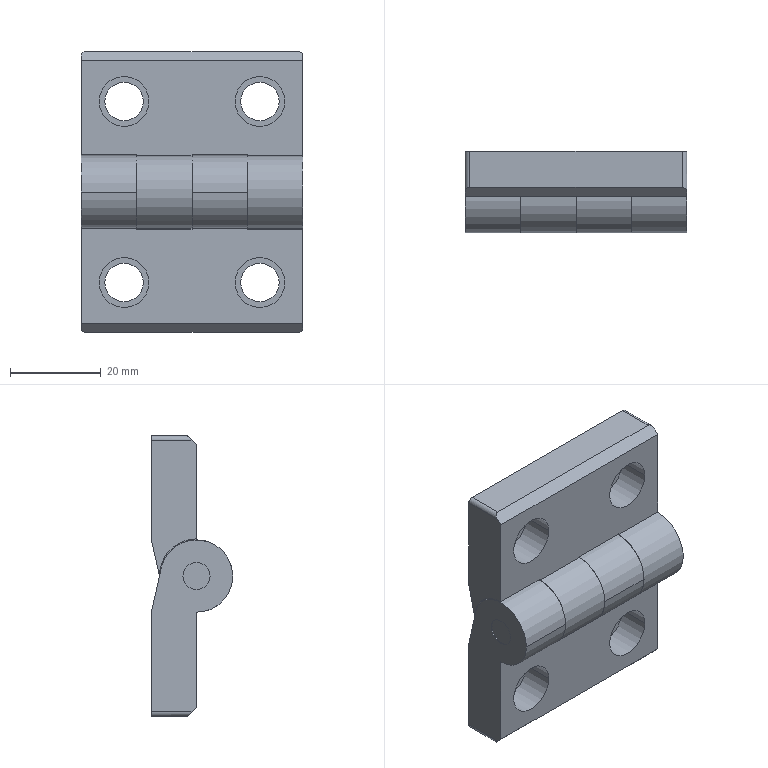Part | SolidWorks | features BaseBody 3 | 3 solids | 66 faces | box 49 x 18 x 62 mm | volume 30925 mm3 | cylinder 40 | plane 26 | commonest cylinder face diameters 6 x10 8.5 x8 11 x8 16 x6 2 x4 16.4 x4